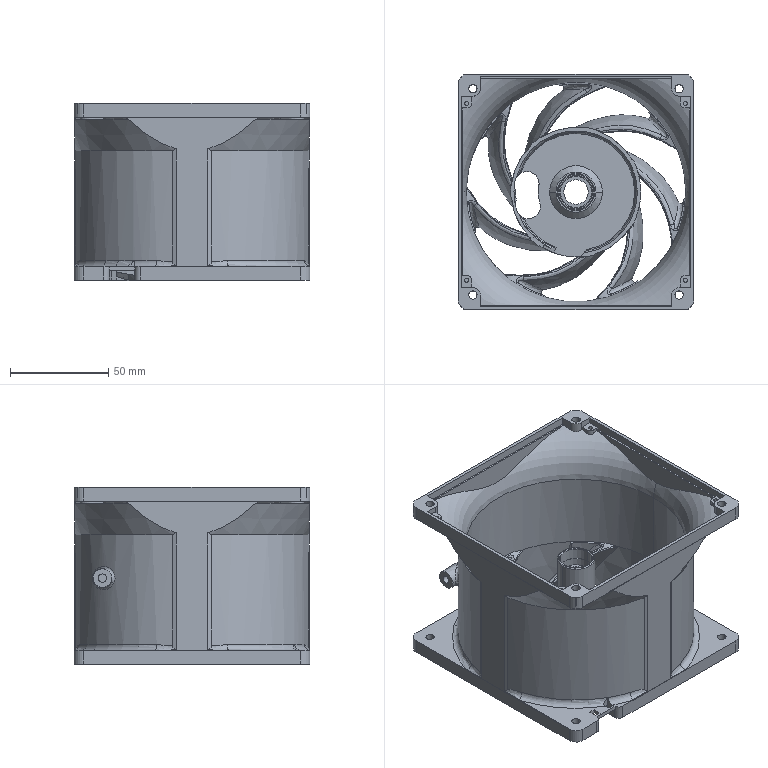Part | 1 solid | 439 faces | box 120 x 120 x 90.2 mm | volume 185382 mm3 | cylinder 172 | plane 145 | spline 82 | cone 25 | torus 15 | commonest cylinder face diameters 1 x31 4.3 x18 9 x17 119.681 x13 2.1 x8 10 x8